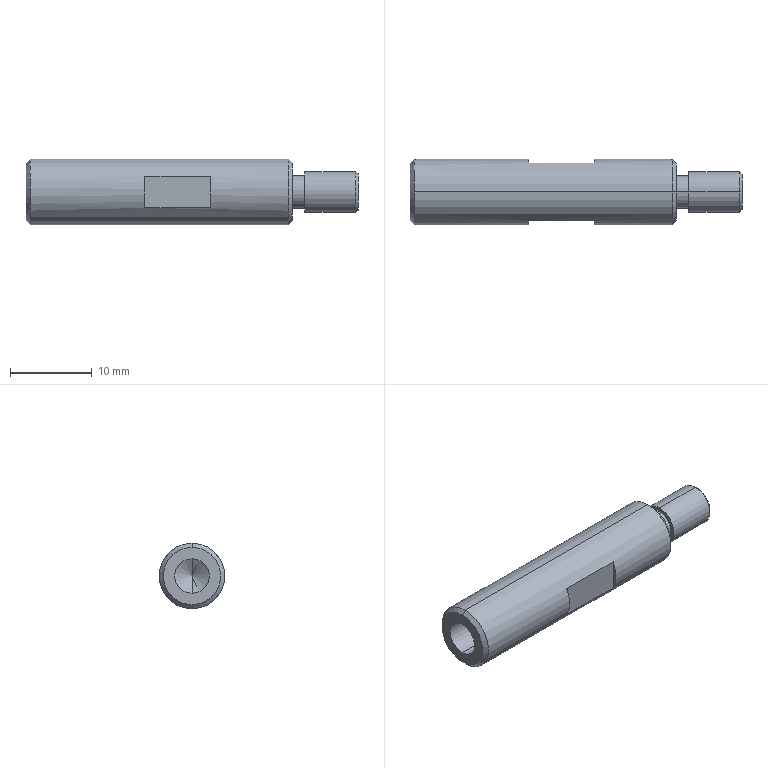Part | STEP file | PN_0016 fixed shaft_Default | 1 solid | 26 faces | box 40.5 x 8 x 8 mm | volume 1575 mm3 | plane 10 | cylinder 8 | cone 8 | commonest cylinder face diameters 4 x2 4.2 x2 5 x2 8 x2